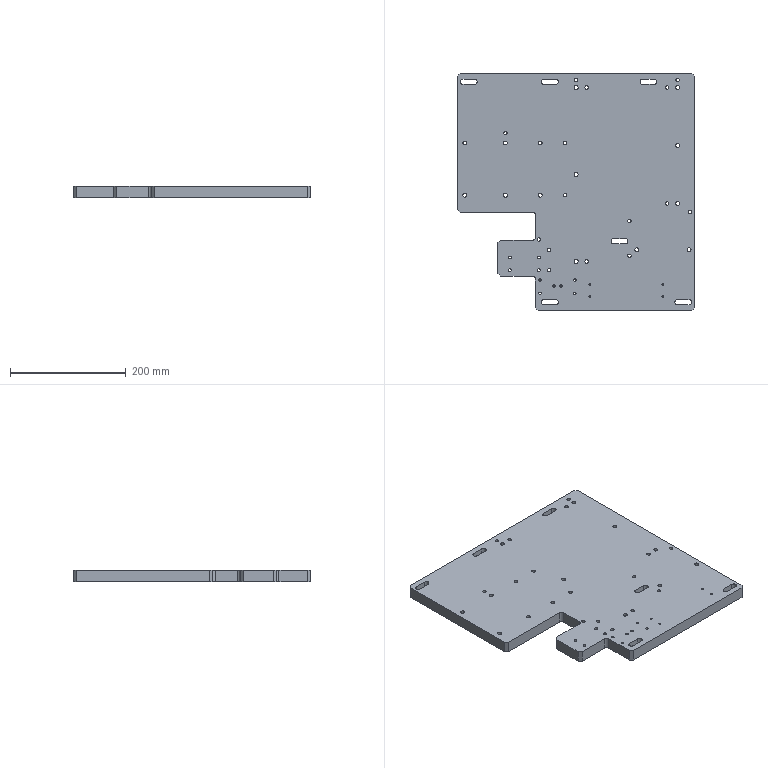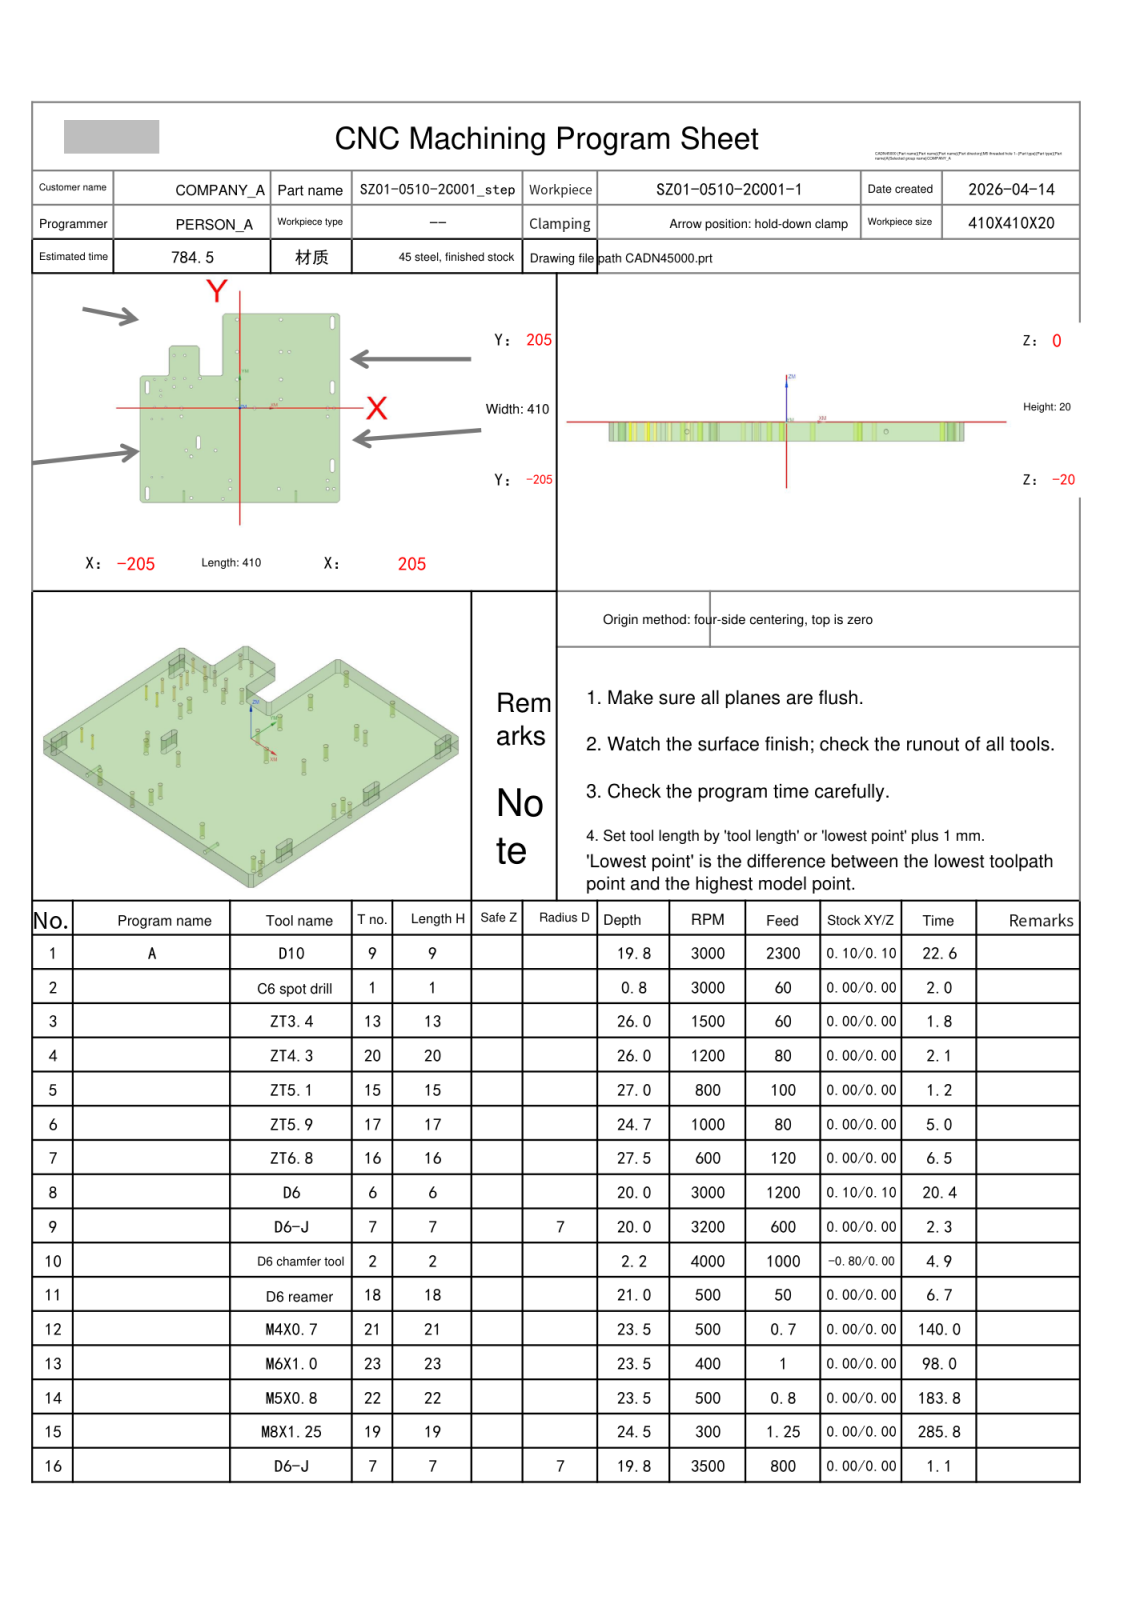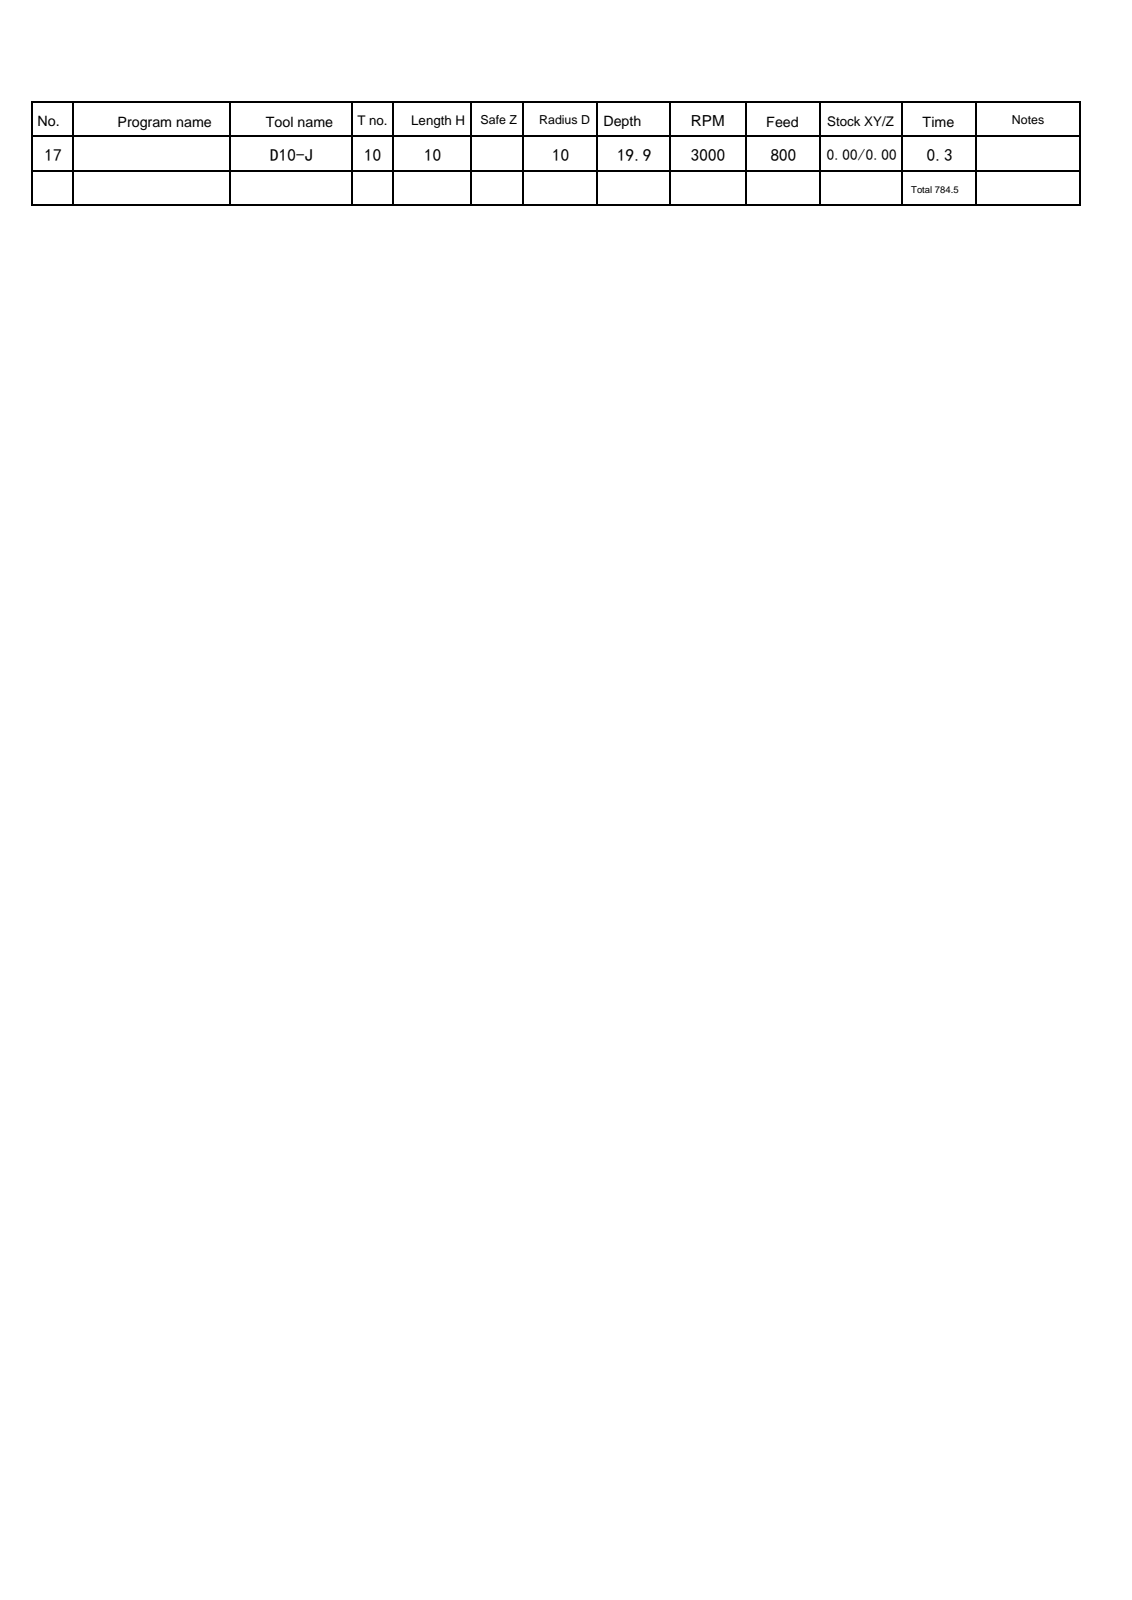NC program | NX | posted by the shop | part box 410 x 410 x 20 mm
Lines 1 to 25 of 7905:
%
O0001
(Machine time: 1466.21 MIN)
(===Total Tool:16===)
(T9=D10     D=10.  R=0.   D-  H09 Z=-19.8 )
(T1=C6 spot drill   D=6.   R=0.   D-  H01 Z=-0.8  )
(T13=ZT3.4  D=3.4  DR_a=118 D-  H13 Z=-26.  )
(T20=ZT4.3  D=4.3  DR_a=118 D-  H20 Z=-26.  )
(T15=ZT5.1  D=5.1  DR_a=118 D-  H15 Z=-27.  )
(T17=ZT5.9  D=5.9  DR_a=120 D-  H17 Z=-24.7 )
(T16=ZT6.8  D=6.8  DR_a=118 D-  H16 Z=-27.54)
(T6=D6      D=6.   R=0.   D-  H06 Z=-20.  )
(T7=D6-J    D=6.   R=0.   D7  H07 Z=-20.  )
(T2=D6 chamfer tool   D=6.   R=0.   D-  H02 Z=-2.2  )
(T18=D6 reamer   D=6.   DR_a=180 D-  H18 Z=-21.  )
(T21=M4X0.7 D=3.3  DR_a=180 D-  H21 Z=-23.5 )
(T23=M6X1.0 D=5.   DR_a=180 D-  H23 Z=-23.5 )
(T22=M5X0.8 D=4.2  DR_a=180 D-  H22 Z=-23.5 )
(T19=M8X1.25 D=6.8  DR_a=180 D-  H19 Z=-24.5 )
(T10=D10-J  D=10.  R=0.   D10 H10 Z=-19.9 )
G80 G90 G17 G49 G40
G91 G28 Z0
M01